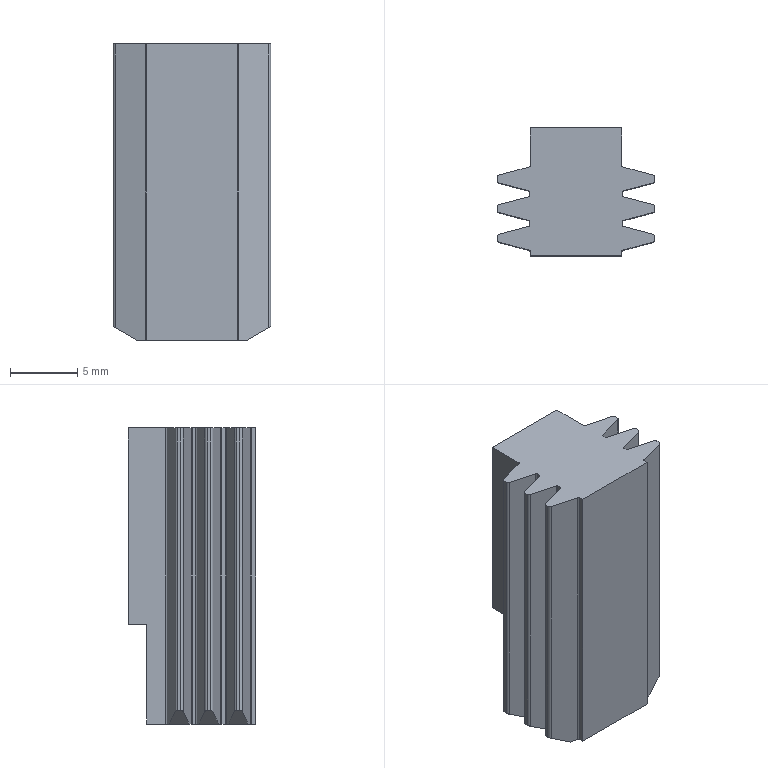Part | SolidWorks | features BaseBody 1 | 1 solid | 82 faces | box 11.68 x 9.5 x 22 mm | volume 1629 mm3 | plane 38 | cylinder 32 | cone 12 | commonest cylinder face diameters 0.2 x12 0.4 x12 2.013 x4 4 x4